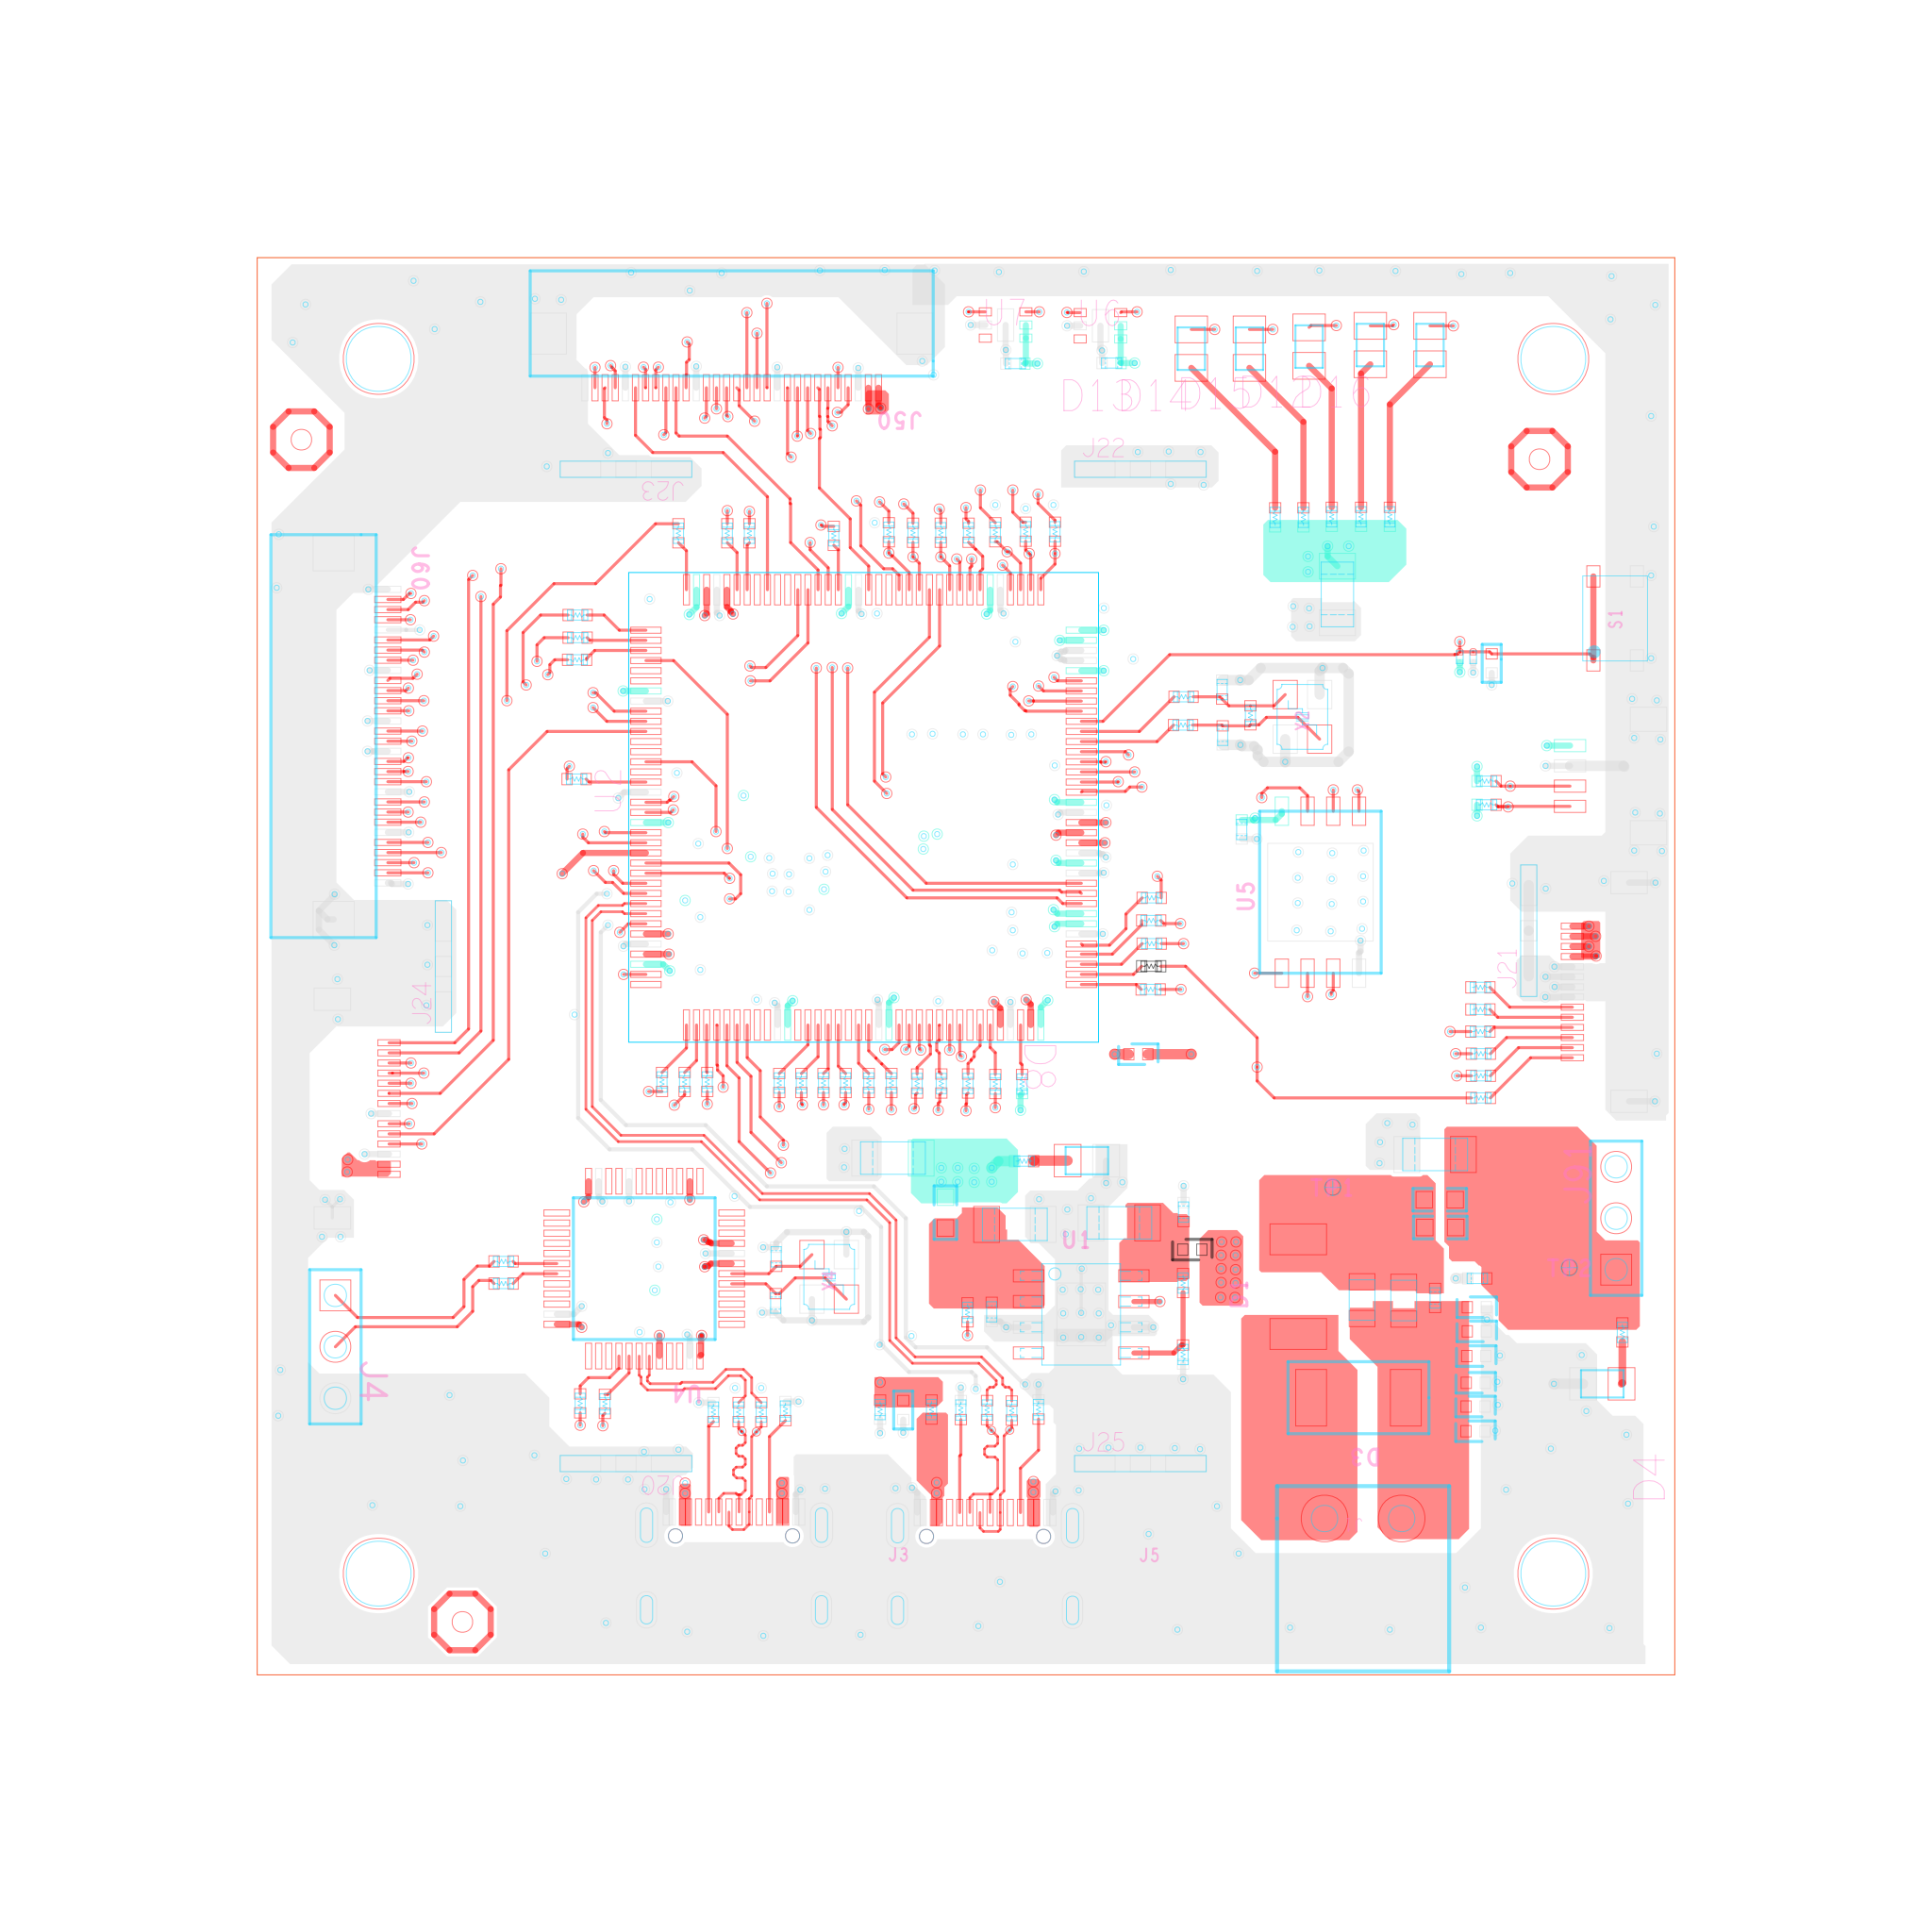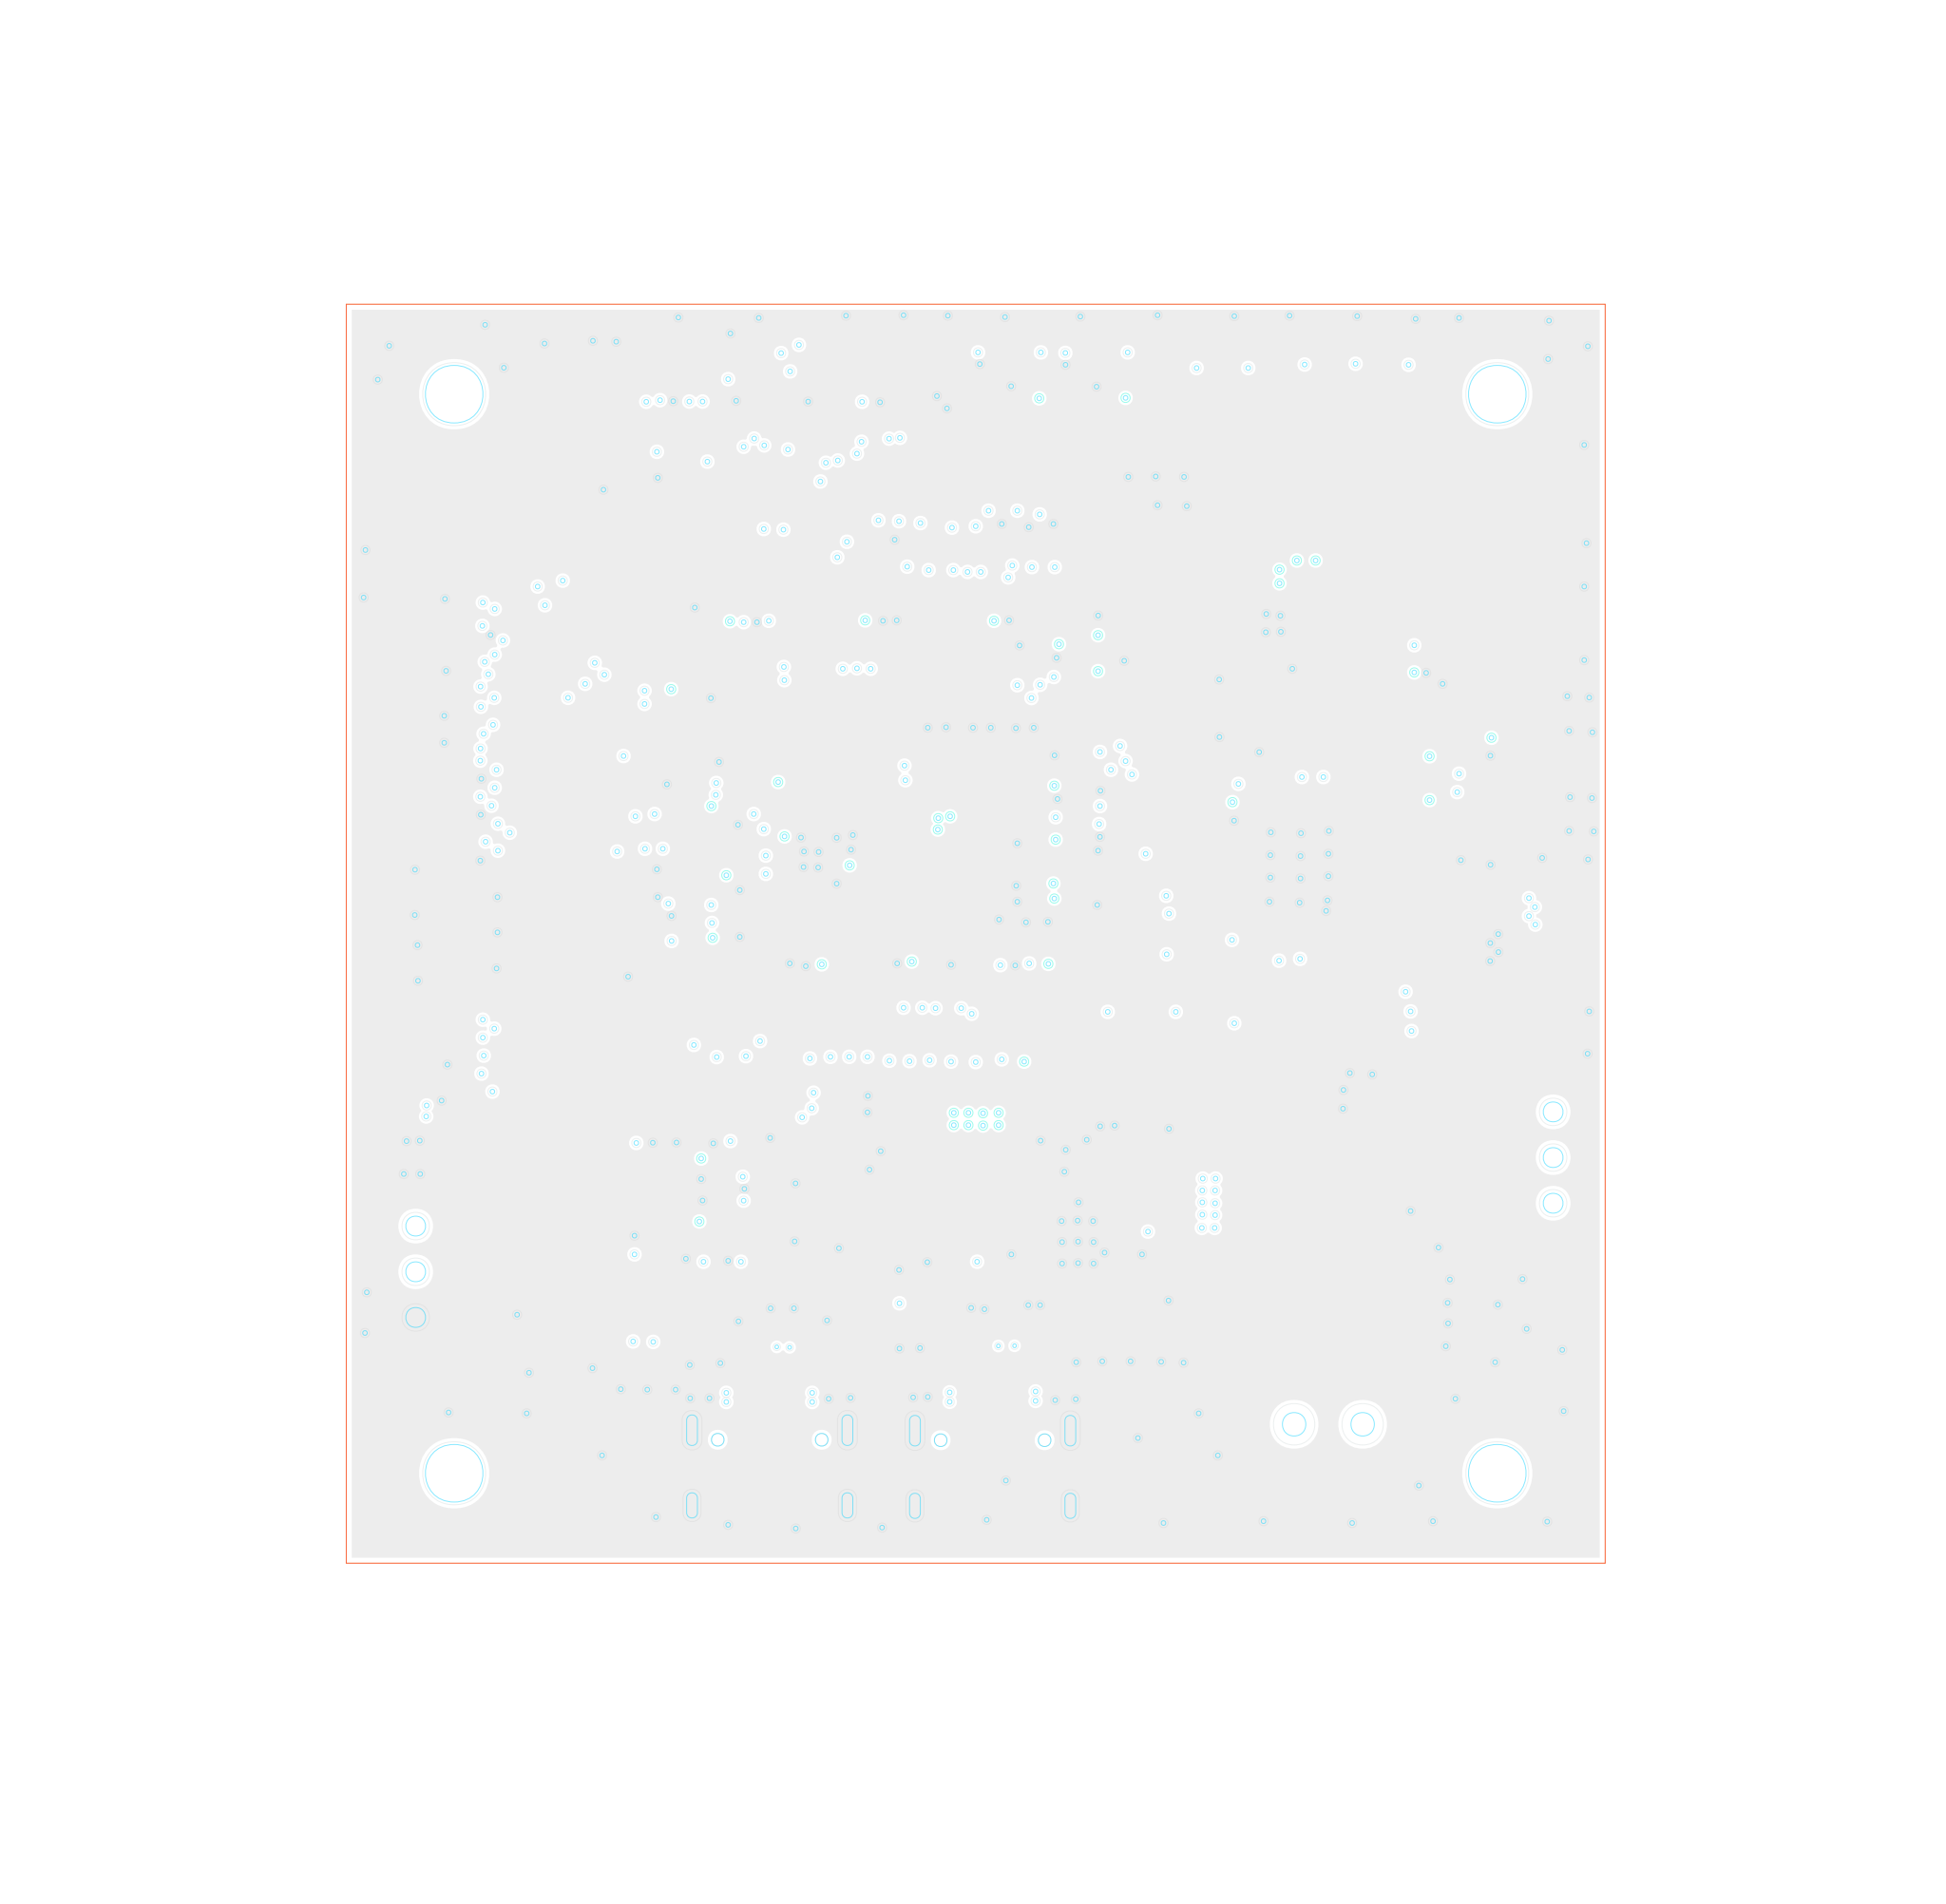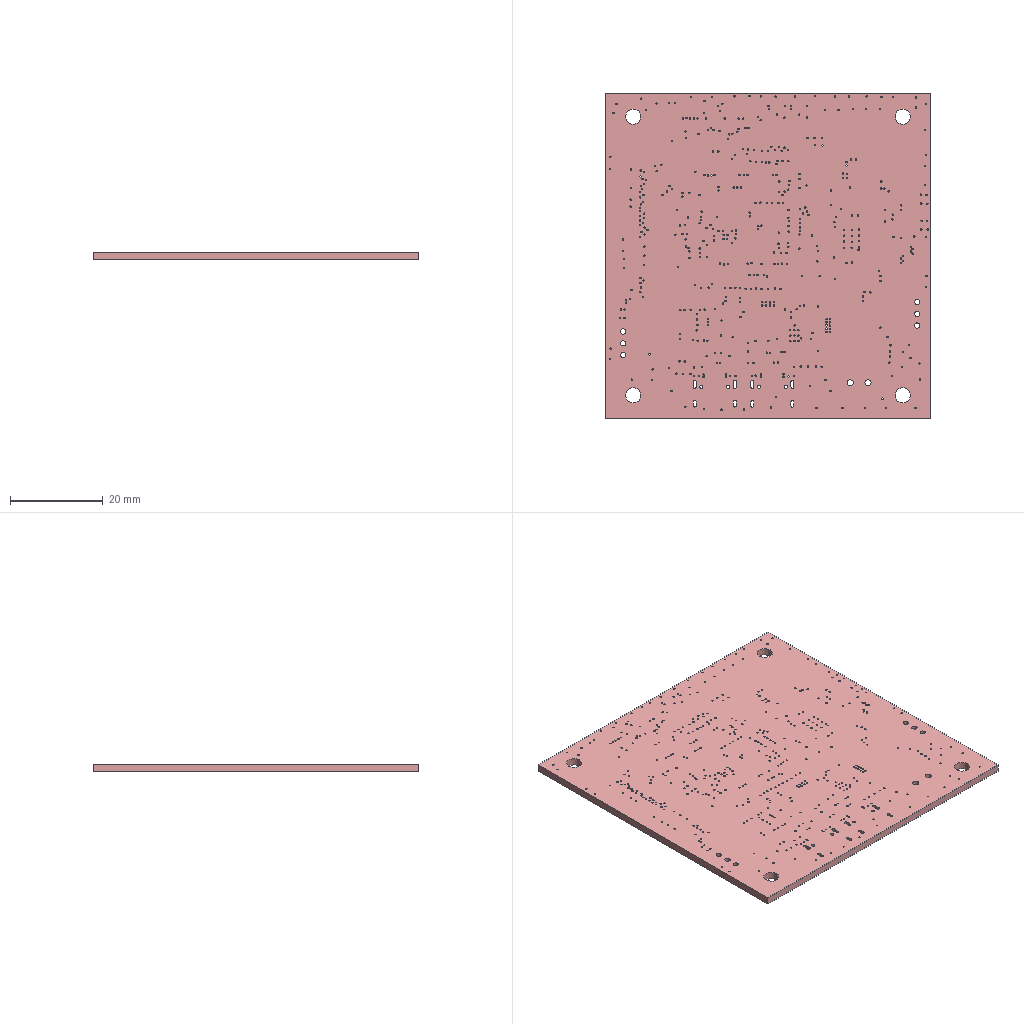Circuit board layout | Cadence Allegro | box 70 x 70 x 1.6 mm
Layer stack:
# Cadence Allegro layer stack of  (unit mm; from the constraint file cross-section; dielectric type: 0 not recorded (Allegro does not mark core vs prepreg), 3 surface material)
index,name,kind,layer,copper_thickness_mm,dielectric_type,dielectric_thickness_mm,dielectric_material,dielectric_constant
0,Top Surface,other,,,,,,
1,Dielectric1,dielectric,,,3,0.0127,FR-4,4.5
2,TOP,copper,TOP,0.0457,,,,
3,Dielectric2,dielectric,,,0,0.0813,FR-4,4.5
4,L2,copper,L2,0.0305,,,,
5,Dielectric3,dielectric,,,0,0.8288,FR-4,4.5
6,L3,copper,L3,0.0305,,,,
7,Dielectric4,dielectric,,,0,0.2032,FR-4,4.5
8,L4,copper,L4,0.0305,,,,
9,Dielectric5,dielectric,,,0,0.2032,FR-4,4.5
10,L5,copper,L5,0.0305,,,,
11,Dielectric6,dielectric,,,0,0.2032,FR-4,4.5
12,BOTTOM,copper,BOTTOM,0.0457,,,,
13,Dielectric7,dielectric,,,3,0.0127,FR-4,4.5
14,Bottom Surface,other,,,,,,
# drill layer pairs: low layer,high layer
drill_pair,TOP,BOTTOM
Part placement:
REFDES,COMP_VALUE,SYM_NAME,SYM_X,SYM_Y,SYM_ROTATE,SYM_MIRROR
C1,10uF,A185_C_1206_H160,6501.00,257.00,180.000,NO
C2,0.1uF,A183_C_0402_H50,6583.00,16.00,180.000,NO
C4,22uF,A186_C_0805_H125,6359.00,-26.00,270.000,NO
C5,22uF,A186_C_0805_H125,6440.00,-27.00,270.000,NO
C6,0.1uF,A183_C_0402_H50,6501.00,-22.00,270.000,NO
C33,10uF,A185_C_1206_H160,5887.00,124.00,180.000,NO
C34,1uF,A183_C_0402_H50,6012.00,145.00,90.000,NO
C35,1uF,A183_C_0402_H50,5639.00,-49.00,270.000,NO
C36,10uF,A185_C_1206_H160,5684.00,121.00,0.000,NO
C59,100nF,A183_C_0402_H50,5721.00,821.00,0.000,YES
C60,100nF,A183_C_0402_H50,5801.00,995.00,270.000,YES
C61,100nF,A183_C_0402_H50,5747.00,606.00,270.000,YES
C62,100nF,A183_C_0402_H50,5636.00,1259.00,90.000,YES
C63,100nF,A183_C_0402_H50,5053.00,594.00,180.000,YES
C64,100nF,A183_C_0402_H50,5366.00,1338.00,180.000,YES
C65,100nF,A183_C_0402_H50,5720.00,741.00,0.000,YES
C66,100nF,A183_C_0402_H50,5887.00,1202.00,270.000,YES
C67,100nF,A183_C_0402_H50,5229.00,582.00,0.000,YES
C83,0.1uF,A454_C_0201_H33,6575.00,1224.00,270.000,NO
C84,0.1uF,A183_C_0402_H50,5054.00,684.00,180.000,YES
C85,0.1uF,A183_C_0402_H50,5127.00,1277.00,0.000,YES
C86,0.1uF,A183_C_0402_H50,5640.00,604.00,270.000,YES
C87,10uF,A185_C_1206_H160,5874.00,631.00,0.000,YES
C88,10uF,A185_C_1206_H160,5873.01,738.00,0.000,YES
C89,220pF,A183_C_0402_H50,5827.00,831.00,90.000,YES
C90,10uF,A185_C_1206_H160,5607.00,978.00,270.000,YES
C91,10uF,A185_C_1206_H160,5702.00,978.00,270.000,YES
C92,10uF,A185_C_1206_H160,5513.00,978.00,270.000,YES
C93,0.1uF,A183_C_0402_H50,5054.00,639.00,180.000,YES
C94,0.1uF,A183_C_0402_H50,5108.00,1338.00,180.000,YES
C95,0.1uF,A183_C_0402_H50,5699.00,607.00,270.000,YES
C96,22uF,A186_C_0805_H125,5229.99,519.00,0.000,YES
C97,10uF,A185_C_1206_H160,5369.01,1262.00,180.000,YES
C98,10uF,A185_C_1206_H160,5447.00,250.00,180.000,NO
C99,2.2uF,A183_C_0402_H50,5430.00,585.00,0.000,YES
C100,100nF,A183_C_0402_H50,5023.00,1337.00,0.000,YES
C101,100nF,A183_C_0402_H50,4968.00,1147.00,180.000,YES
C102,100nF,A183_C_0402_H50,4971.00,927.00,270.000,YES
C103,100nF,A183_C_0402_H50,5070.00,914.00,90.000,YES
C104,100nF,A183_C_0402_H50,5067.00,1002.00,270.000,YES
C105,100nF,A183_C_0402_H50,5727.00,1254.00,0.000,YES
C106,100nF,A183_C_0402_H50,5721.00,693.00,0.000,YES
C107,100nF,A183_C_0402_H50,5885.00,1300.00,270.000,YES
C108,10uF,A185_C_1206_H160,6311.00,1346.00,270.000,NO
C109,18pF,A183_C_0402_H50,6087.00,1161.00,270.000,NO
C110,18pF,A183_C_0402_H50,6088.00,1072.00,90.000,NO
C111,10nF,A183_C_0402_H50,5540.00,1466.00,90.000,YES
C112,10nF,A183_C_0402_H50,5486.00,1466.00,90.000,YES
C113,10nF,A183_C_0402_H50,5440.00,1467.00,90.000,YES
C114,0.1uF,A183_C_0402_H50,5034.00,39.00,0.000,YES
C115,10pF,A183_C_0402_H50,5219.00,-32.00,90.000,NO
C116,10pF,A183_C_0402_H50,5220.00,58.00,270.000,NO
C117,0.1uF,A183_C_0402_H50,5036.00,86.00,0.000,YES
C118,0.1uF,A183_C_0402_H50,4865.00,140.00,180.000,YES
C119,0.1uF,A183_C_0402_H50,5060.00,-120.00,0.000,YES
C120,0.1uF,A183_C_0402_H50,4871.00,-57.00,270.000,YES
C126,1uF,A183_C_0402_H50,6125.00,889.00,270.000,NO
C127,1uF,A183_C_0402_H50,5872.00,1796.00,180.000,NO
C128,1uF,A183_C_0402_H50,5685.00,1795.00,180.000,NO
C139,100nF,A183_C_0402_H50,5188.00,858.00,180.000,YES
C140,10uF,A184_C_0603_H80,5345.00,809.00,270.000,YES
C141,10nF,A183_C_0402_H50,5705.00,1468.00,90.000,YES
C142,10nF,A183_C_0402_H50,5646.00,1467.00,90.000,YES
C143,10nF,A183_C_0402_H50,5762.00,1468.00,90.000,YES
D1,20V,DO_214AA_H244,6235.00,0.00,90.000,NO
D3,15V_600W,A018_DO_214AA_H244,6352.00,-216.00,180.000,NO
D4,LED_SINGLE,LED0805,6826.00,-189.00,90.000,NO
D5,5V,A179_D_0402,5631.00,-239.00,90.000,YES
D6,5V,A179_D_0402,5678.00,-240.00,90.000,YES
D8,LED_SINGLE,LED0805,5824.00,245.00,270.000,NO
D11,5V,A179_D_0402,6611.00,1212.00,90.000,NO
D12,LED_SINGLE,LED0805,6375.00,1831.00,0.000,NO
D13,LED_SINGLE,LED0805,6027.00,1824.00,0.000,NO
D14,LED_SINGLE,LED0805,6140.00,1824.00,0.000,NO
D15,LED_SINGLE,LED0805,6256.00,1828.00,0.000,NO
D16,LED_SINGLE,LED0805,6491.00,1831.00,0.000,NO
D17,5V,A179_D_0402,5147.00,-244.00,90.000,YES
D18,5V,A179_D_0402,5191.00,-244.00,90.000,YES
D19,5V,A179_D_0402,5467.00,-240.00,90.000,NO
FB3,BLM15EG121SN1D,A041_L_0402_H60,5562.00,853.00,0.000,YES
FB4,BLM15EG121SN1D,A041_L_0402_H60,5926.00,400.00,180.000,YES
FB5,BLM15EG121SN1D,A041_L_0402_H60,5724.00,524.00,0.000,YES
FB6,BLM15EG121SN1D,A041_L_0402_H60,5891.00,924.00,270.000,YES
FB7,BLM15EG121SN1D,A041_L_0402_H60,5801.00,907.00,270.000,YES
FB8,BLM15EG121SN1D,A041_L_0402_H60,5924.00,452.00,180.000,YES
FB9,BLM15EG121SN1D,A041_L_0402_H60,5924.00,452.00,0.000,NO
FB10,BLM15EG121SN1D,A041_L_0402_H60,5138.00,978.00,180.000,YES
FB11,BLM15EG121SN1D,A041_L_0402_H60,5138.00,931.00,180.000,YES
J1,WJ15EDGRC-3.81-2P,CON-DZ_2P_3R81,6361.00,-450.88,180.000,NO
J3,KH-TYPE-C-16P,USB-4P-B,5138.01,-533.34,0.000,NO
J4,CON3,HEADER3,4363.00,-117.00,270.000,NO
J5,KH-TYPE-C-16P,USB-4P-B,5626.01,-534.34,0.000,NO
J20,SHIELD_3P,SHIELD_3P,4928.00,-344.00,180.000,NO
J21,SHIELD_3P,SHIELD_3P,6683.00,692.15,90.000,NO
J22,SHIELD_3P,SHIELD_3P,5928.00,1589.50,0.000,NO
J23,SHIELD_3P,SHIELD_3P,4928.00,1589.50,180.000,NO
J24,SHIELD_3P,SHIELD_3P,4573.00,622.50,90.000,NO
J25,SHIELD_3P,SHIELD_3P,5928.00,-344.00,0.000,NO
J40,FPC-05F-14PH15,FPC-05F-14PH15,4412.24,346.31,270.000,NO
J50,FPC-0.5-CON30,FPCS_05PITCH_30P,5133.50,1748.00,180.000,NO
J60,FPC-0.5-CON30,FPCS_05PITCH_30P,4465.00,1070.50,270.000,NO
J91,CON3,HEADER3,6853.00,133.00,90.000,NO
L2,120ohm_100MHz_1.5A,A041_L_0402_H60,6582.00,-40.00,0.000,NO
L3,120ohm_100MHz_1.5A,A041_L_0402_H60,6581.00,-135.00,0.000,NO
L4,120ohm_100MHz_1.5A,A041_L_0402_H60,6582.00,-87.00,0.000,NO
L5,120ohm_100MHz_1.5A,A041_L_0402_H60,6580.00,-187.00,0.000,NO
L6,120ohm_100MHz_1.5A,A041_L_0402_H60,6579.67,-233.15,0.000,NO
L7,120ohm_100MHz_1.5A,A041_L_0402_H60,6579.49,-281.15,0.000,NO
L15,120ohm_100MHz_1.5A,A041_L_0402_H60,6029.00,72.00,180.000,NO
L19,2.2uH,A041_L_0402_RF_H60,5890.00,834.00,90.000,YES
R1,0R,A082_R_0603_H45,6511.00,115.00,0.000,NO
R2,0R,A082_R_0603_H45,6510.00,169.00,0.000,NO
R38,100K,A081_R_0402_H35,6011.00,7.00,270.000,NO
R39,0R,A082_R_0603_H45,5549.00,144.00,90.000,NO
R40,100K,A081_R_0402_H35,5592.00,-49.99,270.000,NO
R41,470R,A081_R_0402_H35,5702.00,244.00,0.000,NO
R46,100K,A081_R_0402_H35,6011.00,-132.00,270.000,NO
R97,10K,A454_C_0201_H33,6549.00,1224.00,270.000,NO
R98,4.7K,A081_R_0402_H35,5098.00,-244.01,90.000,NO
R99,0R,A081_R_0402_H35,5147.00,-243.99,90.000,NO
R100,0R,A081_R_0402_H35,5191.00,-244.00,90.000,NO
R101,4.7K,A081_R_0402_H35,5238.00,-242.00,90.000,NO
R102,100K,A081_R_0402_H35,6865.00,-89.00,270.000,NO
R103,470R,A081_R_0402_H35,6357.00,1497.00,90.000,NO
R104,470R,A081_R_0402_H35,6190.00,1496.00,90.000,NO
R105,470R,A081_R_0402_H35,6245.00,1496.00,90.000,NO
R106,470R,A081_R_0402_H35,6300.00,1497.00,90.000,NO
R107,470R,A081_R_0402_H35,6413.00,1497.00,90.000,NO
R108,0R,A082_R_0603_H45,5937.00,346.00,180.000,YES
R109,10K,A081_R_0402_H35,5698.00,394.00,90.000,NO
R110,10K,A081_R_0402_H35,5557.00,508.00,90.000,YES
R111,1M,A081_R_0402_H35,6142.00,1111.00,270.000,NO
R112,0R,A081_R_0402_H35,6012.00,1147.00,180.000,NO
R113,0R,A081_R_0402_H35,6011.00,1092.00,180.000,NO
R114,33.2R,A081_R_0402_H35,5540.00,1466.00,270.000,NO
R115,33.2R,A081_R_0402_H35,5486.00,1466.00,270.000,NO
R116,33.2R,A081_R_0402_H35,5439.00,1467.00,270.000,NO
R117,0R,A081_R_0402_H35,5949.00,623.00,0.000,NO
R118,33.2R,A081_R_0402_H35,5030.00,1465.00,90.000,NO
R119,33.2R,A081_R_0402_H35,4834.00,1306.00,180.000,NO
R120,33.2R,A081_R_0402_H35,4833.01,1219.00,180.000,NO
R121,33.2R,A081_R_0402_H35,5950.00,756.00,0.000,NO
R122,33.2R,A081_R_0402_H35,5950.00,667.00,0.000,NO
R123,33.2R,A081_R_0402_H35,5948.01,578.00,0.000,NO
R124,33.2R,A081_R_0402_H35,4832.00,987.00,0.000,NO
R125,33.2R,A081_R_0402_H35,5444.00,396.00,90.000,NO
R126,33.2R,A081_R_0402_H35,5400.00,396.01,90.000,NO
R127,33.2R,A081_R_0402_H35,5594.00,1466.00,270.000,NO
R128,33.2R,A081_R_0402_H35,5086.00,398.00,90.000,NO
R129,33.2R,A081_R_0402_H35,4998.00,397.99,90.000,NO
R130,33.2R,A081_R_0402_H35,5494.00,394.99,270.000,NO
R131,33.2R,A081_R_0402_H35,5541.00,395.00,270.000,NO
R132,4.7K,A081_R_0402_H35,5034.00,-7.00,180.000,YES
R134,4.7K,A081_R_0402_H35,4973.00,-120.00,0.000,YES
R135,0R,A081_R_0402_H35,4690.01,6.00,180.000,NO
R136,0R,A081_R_0402_H35,4689.99,49.00,180.000,NO
R137,0R,A081_R_0402_H35,4887.00,-228.00,270.000,NO
R138,0R,A081_R_0402_H35,4839.00,-227.00,270.000,NO
R139,0R,A081_R_0402_H35,5034.00,131.00,180.000,YES
R140,0R,A081_R_0402_H35,5630.00,-240.01,90.000,NO
R141,0R,A081_R_0402_H35,5678.00,-240.99,90.000,NO
R142,4.7K,A081_R_0402_H35,5579.00,-240.00,90.000,NO
R143,4.7K,A081_R_0402_H35,5730.00,-239.00,90.000,NO
R144,1K,A081_R_0402_H35,5522.00,-239.00,90.000,NO
R145,1K,A081_R_0402_H35,5422.00,-239.00,270.000,NO
R153,10K,A081_R_0402_H35,5087.00,794.00,180.000,YES
R154,10K,A081_R_0402_H35,5087.00,751.00,180.000,YES
R155,10K,A081_R_0402_H35,5087.00,838.00,0.000,YES
R156,4.7K,A081_R_0402_H35,5033.00,192.00,180.000,YES
R157,33.2R,A081_R_0402_H35,5949.00,712.00,180.000,NO
R158,33.2R,A081_R_0402_H35,5332.00,1460.00,270.000,NO
R159,0R,A081_R_0402_H35,5593.00,395.00,270.000,NO
R160,0R,A081_R_0402_H35,5646.00,394.00,270.000,NO
R161,100K,A081_R_0402_H35,6601.00,937.00,0.000,NO
R162,100K,A081_R_0402_H35,6601.00,983.00,0.000,NO
R164,33.2R,A081_R_0402_H35,4834.00,1262.00,180.000,NO
R165,33.2R,A081_R_0402_H35,5269.00,395.99,90.000,NO
R166,33.2R,A081_R_0402_H35,5312.00,396.01,90.000,NO
R167,33.2R,A081_R_0402_H35,5355.00,396.00,90.000,NO
R168,33.2R,A081_R_0402_H35,5226.00,396.00,90.000,NO
R169,33.2R,A081_R_0402_H35,5705.00,1468.00,270.000,NO
R170,33.2R,A081_R_0402_H35,5646.00,1467.01,270.000,NO
R171,33.2R,A081_R_0402_H35,5762.00,1467.99,270.000,NO
R172,33.2R,A081_R_0402_H35,5042.00,398.00,90.000,NO
R173,33.2R,A081_R_0402_H35,6590.00,367.00,0.000,NO
R174,33.2R,A081_R_0402_H35,6590.00,410.00,0.000,NO
R175,0R,A081_R_0402_H35,6589.00,496.00,0.000,NO
R176,0R,A081_R_0402_H35,6590.00,453.00,0.000,NO
R177,33.2R,A081_R_0402_H35,6589.00,539.00,0.000,NO
R178,33.2R,A081_R_0402_H35,6589.00,582.00,0.000,NO
R179,0R,A081_R_0402_H35,5168.00,1464.99,90.000,NO
R180,0R,A081_R_0402_H35,5125.00,1465.01,90.000,NO
S1,SW PUSHBUTTON_4P_A,SW_4-2P15-4P2X3P2-2P5,6850.98,1299.43,90.000,NO
TP1,SMD_HOLE_30C,Z055_TPS_30C,6302.00,193.00,0.000,NO
TP2,SMD_HOLE_30C,Z055_TPS_30C,6762.00,37.00,0.000,NO
U1,ADP7104ARDZ-3.3,RD-8-2,5813.00,-54.00,0.000,NO
U2,STM32H745ZIT6,QFP144-20X20-NO_PAD,5390.00,932.00,90.000,NO
U3,24AA64T-I/MS,DFN8_2X3X1P1,5227.50,782.50,0.000,YES
U4,CH344Q,LQFP48-900X900-H160,4963.50,35.00,180.000,NO
U5,128Mbit_WSON_8X6,A122_VFDFPN8_T_S800X600_H85,6278.00,767.00,90.000,NO
U6,TMP117AIDRVR,WSON6_2X2,5850.37,1868.48,0.000,NO
U7,TMP117AIDRVR,WSON6_2X2,5666.00,1870.00,0.000,NO
U8,SM04B-SRSS-TB,SM04B-SRSS-TB,6839.54,993.00,90.000,NO
U9,FPC-05F-14PH15,FPC-05F-14PH15,6822.97,573.00,90.000,NO
X2,25MHz,X3225,6243.00,1108.00,90.000,NO
X4,8MHz,X3225,5323.00,19.00,90.000,NO
Pad and via stacks, first 111 of 219 lines:
# Allegro (Cadence) via spans and padstacks; design units: ("mils" 2 100)
# via spans: padstack,start_layer,end_layer,net_example,count
VIA8_16-BGA-FULL-NEW,ETCH/TOP,ETCH/BOTTOM,D+,4
VIA20D10,ETCH/TOP,ETCH/BOTTOM,GND,524
# Allegro padstack definitions: name,start_layer,end_layer,drill,plating,holeType,type
BALL0_4-S0_1,"ETCH/TOP","ETCH/TOP",0.0,"PLATED","none","smd"
BALL12,"ETCH/TOP","ETCH/TOP",0.0,"PLATED","none","smd"
S36X16S,"ETCH/TOP","ETCH/TOP",0.0,"PLATED","none","smd"
S50X40S,"ETCH/TOP","ETCH/TOP",0.0,"PLATED","none","smd"
S32S,"ETCH/TOP","ETCH/TOP",0.0,"PLATED","none","smd"
S205X190S,"ETCH/TOP","ETCH/TOP",0.0,"PLATED","none","smd"
S55X26S,"ETCH/TOP","ETCH/TOP",0.0,"PLATED","none","smd"
S22X20S,"ETCH/TOP","ETCH/TOP",0.0,"PLATED","none","smd"
SMD100X200,"ETCH/TOP","ETCH/TOP",0.0,"PLATED","none","smd"
SMD025X180,"ETCH/TOP","ETCH/TOP",0.0,"NON_PLATED","none","smd"
PAD94,"ETCH/TOP","ETCH/TOP",0.0,"NON_PLATED","none","smd"
SQU450,"ETCH/TOP","ETCH/TOP",0.0,"PLATED","none","smd"
OLB030X080,"ETCH/TOP","ETCH/TOP",0.0,"PLATED","none","smd"
S71X44S,"ETCH/TOP","ETCH/TOP",0.0,"NON_PLATED","none","smd"
STP_C30,"ETCH/TOP","ETCH/TOP",0.0,"PLATED","none","smd"
S87X32S,"ETCH/TOP","ETCH/TOP",0.0,"NON_PLATED","none","smd"
SMD60_36-P1,"ETCH/TOP","ETCH/TOP",0.0,"PLATED","none","smd"
SMD8_28,"ETCH/TOP","ETCH/TOP",0.0,"PLATED","none","smd"
S012S,"ETCH/TOP","ETCH/TOP",0.0,"PLATED","none","smd"
S32X26S,"ETCH/TOP","ETCH/TOP",0.0,"PLATED","none","smd"
S40X27S,"ETCH/TOP","ETCH/TOP",0.0,"PLATED","none","smd"
R2M75X3M30,"ETCH/TOP","ETCH/TOP",0.0,"PLATED","none","smd"
R0M40X1M35,"ETCH/TOP","ETCH/TOP",0.0,"PLATED","none","smd"
OBLG020X050,"ETCH/TOP","ETCH/TOP",0.0,"PLATED","none","smd"
OBLG020X070,"ETCH/TOP","ETCH/TOP",0.0,"PLATED","none","smd"
SMD060X110,"ETCH/TOP","ETCH/TOP",0.0,"PLATED","none","smd"
SHAPE030,"ETCH/TOP","ETCH/TOP",0.0,"PLATED","none","smd"
SMD250X280,"ETCH/TOP","ETCH/TOP",0.0,"PLATED","none","smd"
SMD021X0465,"ETCH/TOP","ETCH/TOP",0.0,"NON_PLATED","none","smd"
SMD021X0565,"ETCH/TOP","ETCH/TOP",0.0,"PLATED","none","smd"
C030,"ETCH/TOP","ETCH/TOP",0.0,"PLATED","none","smd"
VIA1-02,"ETCH/TOP","ETCH/L2",4.0,"PLATED","circle_drill","bbvia"
S70X50S,"ETCH/TOP","ETCH/TOP",0.0,"PLATED","none","smd"
S80X70S,"ETCH/TOP","ETCH/TOP",0.0,"PLATED","none","smd"
S51X12S,"ETCH/TOP","ETCH/TOP",0.0,"NON_PLATED","none","smd"
SMD040X160,"ETCH/TOP","ETCH/TOP",0.0,"PLATED","none","smd"
SMD080X170,"ETCH/TOP","ETCH/TOP",0.0,"PLATED","none","smd"
R07S120MM,"ETCH/TOP","ETCH/TOP",0.0,"NON_PLATED","none","smd"
SMD3_6X3_6-MM,"ETCH/TOP","ETCH/TOP",0.0,"PLATED","none","smd"
SMD33_8OB,"ETCH/TOP","ETCH/TOP",0.0,"PLATED","none","smd"
SMD8_33OB,"ETCH/TOP","ETCH/TOP",0.0,"PLATED","none","smd"
SMD050X150,"ETCH/TOP","ETCH/TOP",0.0,"PLATED","none","smd"
SMD100X150,"ETCH/TOP","ETCH/TOP",0.0,"PLATED","none","smd"
R1M80_2M00,"ETCH/TOP","ETCH/TOP",0.0,"PLATED","none","smd"
R0M4_1M25,"ETCH/TOP","ETCH/TOP",0.0,"PLATED","none","smd"
R076S152MM,"ETCH/TOP","ETCH/TOP",0.0,"NON_PLATED","none","smd"
SMD070X160,"ETCH/TOP","ETCH/TOP",0.0,"PLATED","none","smd"
SMD210X300,"ETCH/TOP","ETCH/TOP",0.0,"PLATED","none","smd"
SMD035X050,"ETCH/TOP","ETCH/TOP",0.0,"NON_PLATED","none","smd"
SMD0_254X0_675,"ETCH/TOP","ETCH/TOP",0.0,"PLATED","none","smd"
SMD0_4X1_55,"ETCH/TOP","ETCH/TOP",0.0,"PLATED","none","smd"
R0P2X0P7,"ETCH/TOP","ETCH/TOP",0.0,"NON_PLATED","none","smd"
S150,"ETCH/TOP","ETCH/TOP",0.0,"NON_PLATED","none","smd"
PAD5035,"ETCH/TOP","ETCH/TOP",0.0,"NON_PLATED","none","smd"
R018X020S,"ETCH/TOP","ETCH/TOP",0.0,"PLATED","none","smd"
R028X033S,"ETCH/TOP","ETCH/TOP",0.0,"PLATED","none","smd"
S90X50S,"ETCH/TOP","ETCH/TOP",0.0,"PLATED","none","smd"
S65X60S,"ETCH/TOP","ETCH/TOP",0.0,"PLATED","none","smd"
S63X30S,"ETCH/TOP","ETCH/TOP",0.0,"PLATED","none","smd"
S65X50S,"ETCH/TOP","ETCH/TOP",0.0,"PLATED","none","smd"
S63X32S,"ETCH/TOP","ETCH/TOP",0.0,"PLATED","none","smd"
S120X90S,"ETCH/TOP","ETCH/TOP",0.0,"PLATED","none","smd"
SMD040X100,"ETCH/TOP","ETCH/TOP",0.0,"NON_PLATED","none","smd"
SMD030X160,"ETCH/TOP","ETCH/TOP",0.0,"NON_PLATED","none","smd"
SMD180X080,"ETCH/TOP","ETCH/TOP",0.0,"PLATED","none","smd"
SMD030X120,"ETCH/TOP","ETCH/TOP",0.0,"PLATED","none","smd"
SMD10_30OB,"ETCH/TOP","ETCH/TOP",0.0,"PLATED","none","smd"
SMD30_10OB,"ETCH/TOP","ETCH/TOP",0.0,"PLATED","none","smd"
SMD138_138-TNP,"ETCH/TOP","ETCH/TOP",0.0,"PLATED","none","smd"
PAD1,"ETCH/TOP","ETCH/TOP",0.0,"NON_PLATED","none","smd"
SMD030X160-2222222,"ETCH/TOP","ETCH/TOP",0.0,"NON_PLATED","none","smd"
SMD025X040,"ETCH/TOP","ETCH/TOP",0.0,"NON_PLATED","none","smd"
SMD025X065,"ETCH/TOP","ETCH/TOP",0.0,"PLATED","none","smd"
SMD055X080-1,"ETCH/TOP","ETCH/TOP",0.0,"PLATED","none","smd"
SMD070X140,"ETCH/TOP","ETCH/TOP",0.0,"PLATED","none","smd"
SMD060X095,"ETCH/TOP","ETCH/TOP",0.0,"NON_PLATED","none","smd"
CIR035,"ETCH/TOP","ETCH/TOP",0.0,"NON_PLATED","none","smd"
VIA06-07,"ETCH/L3","ETCH/L3",4.0,"PLATED","circle_drill","bbvia"
VIA03-06,,,8.0,"PLATED","circle_drill","through"
VIA02-07,"ETCH/L2","ETCH/L3",8.0,"PLATED","circle_drill","bbvia"
R0P7X1P25,"ETCH/TOP","ETCH/TOP",0.0,"PLATED","none","smd"
SMD25_20,"ETCH/TOP","ETCH/TOP",0.0,"PLATED","none","smd"
SMD050,"ETCH/TOP","ETCH/TOP",0.0,"PLATED","none","smd"
SMD140_165,"ETCH/TOP","ETCH/TOP",0.0,"NON_PLATED","none","smd"
R1P4X1P2,"ETCH/TOP","ETCH/TOP",0.0,"NON_PLATED","none","smd"
SMD060X150,"ETCH/TOP","ETCH/TOP",0.0,"PLATED","none","smd"
SMD3_1X2_4-MM,"ETCH/TOP","ETCH/TOP",0.0,"PLATED","none","smd"
SMT052X063,"ETCH/TOP","ETCH/TOP",0.0,"PLATED","none","smd"
S75X60S,"ETCH/TOP","ETCH/TOP",0.0,"PLATED","none","smd"
S55X16S,"ETCH/TOP","ETCH/TOP",0.0,"PLATED","none","smd"
R1P05X0P65,"ETCH/TOP","ETCH/TOP",0.0,"NON_PLATED","none","smd"
R0P3X1P45,"ETCH/TOP","ETCH/TOP",0.0,"NON_PLATED","none","smd"
SMDR220X60,"ETCH/TOP","ETCH/TOP",0.0,"PLATED","none","smd"
SMD035X135,"ETCH/TOP","ETCH/TOP",0.0,"PLATED","none","smd"
S50X12S,"ETCH/TOP","ETCH/TOP",0.0,"PLATED","none","smd"
SMD030X085,"ETCH/TOP","ETCH/TOP",0.0,"PLATED","none","smd"
S65X13S,"ETCH/TOP","ETCH/TOP",0.0,"PLATED","none","smd"
SMD025X155,"ETCH/TOP","ETCH/TOP",0.0,"PLATED","none","smd"
SMD155X250,"ETCH/TOP","ETCH/TOP",0.0,"PLATED","none","smd"
SMD205X250,"ETCH/TOP","ETCH/TOP",0.0,"PLATED","none","smd"
SMD130X155,"ETCH/TOP","ETCH/TOP",0.0,"NON_PLATED","none","smd"
VIA07-08,"ETCH/L3","ETCH/BOTTOM",4.0,"PLATED","circle_drill","bbvia"
VIA10-BGA-FULL,"ETCH/TOP","ETCH/BOTTOM",10.0,"PLATED","circle_drill","through"
VIA8_16-BGA-FULL-NEW,"ETCH/TOP","ETCH/BOTTOM",8.0,"PLATED","circle_drill","through"
HOLE0P60,"ETCH/TOP","ETCH/BOTTOM",23.62,"NON_PLATED","circle_drill","through"
SPAD050-1000,"ETCH/TOP","ETCH/BOTTOM",19.69,"PLATED","circle_drill","through"
Design rules, without the lines most boards share, first 8 of 51 lines:
# Cadence Allegro design rules of  (from the Constraint Manager export constraints.dcfx, design unit mil; typed fields in mm)
# columns: name | kind | enabled | priority | scope1 | scope2 | descriptor | typed fields (field=value)
# Allegro precedence (priority 1 wins): 1 Region class-to-class, 2 Region class, 3 Region, 4 class-to-class, 5 DiffPair/Bus/NetGroup override, 6 NetClass, 7 constraint set (CSet) default
# per-layer values are written LAYER=value in the descriptor and LAYER:mm in the typed field; a maximum of 0 means no limit set
# --- net classes (and buses / net groups) ---
DIFF100 | NetClass | enabled | 6 | no members | All | Net Class (PhysicalCSet=DIFF100) (SpacingCSet=15) (members: 0) | physicalcset=DIFF100 spacingcset=15
POWER | NetClass | enabled | 6 | no members | All | Net Class (PhysicalCSet=POWER) (members: 0) | physicalcset=POWER
SOC2CAM_MIPI0 | NetClass | enabled | 6 | no members | All | Net Class (members: 0) |